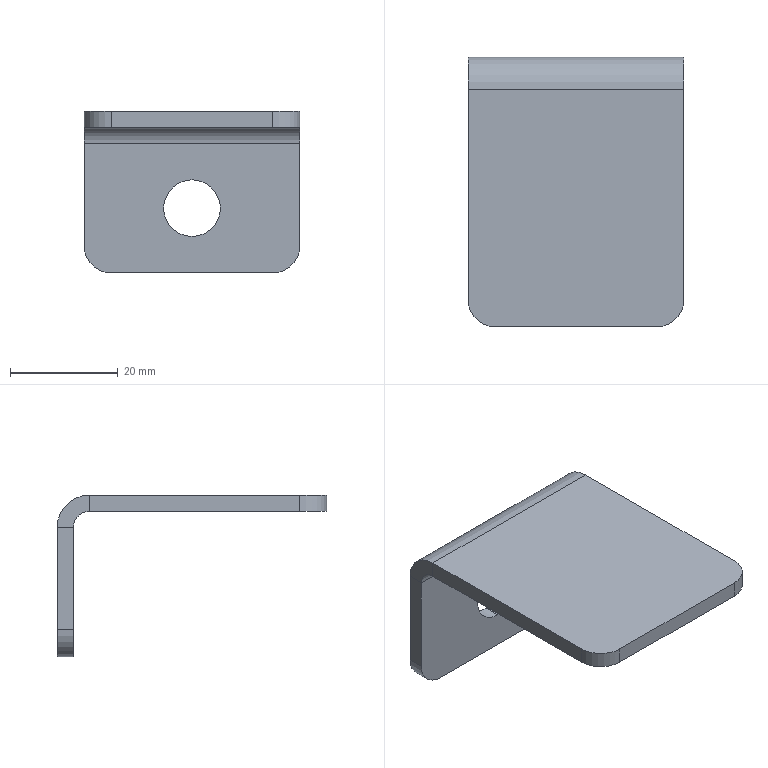Part | SolidWorks | features EdgeFlange 1, Fillet 1, FlatPattern 1, ICE 1, SMBaseFlange 1, SheetMetal 1 | 1 solid | 20 faces | box 40 x 50 x 30 mm | volume 8684 mm3 | plane 12 | cylinder 8 | commonest cylinder face diameters 10 x4 10.5 x2 6 x1 12 x1
STEP:
#1=CARTESIAN_POINT('',(0.,22.,-23.25));
#2=VERTEX_POINT('',#1);
#3=CARTESIAN_POINT('',(0.,22.,-12.75));
#4=VERTEX_POINT('',#3);
#5=CARTESIAN_POINT('',(0.,22.,-18.));
#6=DIRECTION('',(0.,1.,0.));
#7=DIRECTION('',(0.,0.,1.));
#8=AXIS2_PLACEMENT_3D('',#5,#6,#7);
#9=CIRCLE('',#8,5.25);
#10=EDGE_CURVE('',#2,#4,#9,.T.);
#11=ORIENTED_EDGE('',*,*,#10,.F.);
#12=CARTESIAN_POINT('',(0.,25.,-23.25));
#13=VERTEX_POINT('',#12);
#14=CARTESIAN_POINT('',(0.,15.,-23.25));
#15=DIRECTION('',(0.,1.,0.));
#16=VECTOR('',#15,1000.);
#17=LINE('',#14,#16);
#18=EDGE_CURVE('',#2,#13,#17,.T.);
#19=ORIENTED_EDGE('',*,*,#18,.T.);
#20=CARTESIAN_POINT('',(0.,25.,-12.75));
#21=VERTEX_POINT('',#20);
#22=CARTESIAN_POINT('',(0.,25.,-18.));
#23=DIRECTION('',(0.,1.,0.));
#24=DIRECTION('',(0.,0.,1.));
#25=AXIS2_PLACEMENT_3D('',#22,#23,#24);
#26=CIRCLE('',#25,5.25);
#27=EDGE_CURVE('',#13,#21,#26,.T.);
#28=ORIENTED_EDGE('',*,*,#27,.T.);
#29=CARTESIAN_POINT('',(0.,15.,-12.75));
#30=DIRECTION('',(0.,1.,0.));
#31=VECTOR('',#30,1000.);
#32=LINE('',#29,#31);
#33=EDGE_CURVE('',#4,#21,#32,.T.);
#34=ORIENTED_EDGE('',*,*,#33,.F.);
#35=EDGE_LOOP('',(#11,#19,#28,#34));
#36=FACE_OUTER_BOUND('',#35,.T.);
#37=CARTESIAN_POINT('',(0.,15.,-18.));
#38=DIRECTION('',(0.,1.,0.));
#39=DIRECTION('',(0.,0.,1.));
#40=AXIS2_PLACEMENT_3D('',#37,#38,#39);
#41=CYLINDRICAL_SURFACE('',#40,5.25);
#42=ADVANCED_FACE('',(#36),#41,.F.);
#43=CARTESIAN_POINT('',(20.,-20.,0.));
#44=VERTEX_POINT('',#43);
#45=CARTESIAN_POINT('',(20.,19.,0.));
#46=VERTEX_POINT('',#45);
#47=CARTESIAN_POINT('',(20.,25.,0.));
#48=DIRECTION('',(0.,1.,0.));
#49=VECTOR('',#48,1000.);
#50=LINE('',#47,#49);
#51=EDGE_CURVE('',#44,#46,#50,.T.);
#52=ORIENTED_EDGE('',*,*,#51,.F.);
#53=CARTESIAN_POINT('',(20.,-20.,-3.));
#54=VERTEX_POINT('',#53);
#55=CARTESIAN_POINT('',(20.,-20.,-3.));
#56=DIRECTION('',(0.,0.,-1.));
#57=VECTOR('',#56,1000.);
#58=LINE('',#55,#57);
#59=EDGE_CURVE('',#44,#54,#58,.T.);
#60=ORIENTED_EDGE('',*,*,#59,.T.);
#61=CARTESIAN_POINT('',(20.,19.,-3.));
#62=VERTEX_POINT('',#61);
#63=CARTESIAN_POINT('',(20.,25.,-3.));
#64=DIRECTION('',(0.,1.,0.));
#65=VECTOR('',#64,1000.);
#66=LINE('',#63,#65);
#67=EDGE_CURVE('',#54,#62,#66,.T.);
#68=ORIENTED_EDGE('',*,*,#67,.T.);
#69=CARTESIAN_POINT('',(20.,19.,-3.));
#70=DIRECTION('',(0.,0.,1.));
#71=VECTOR('',#70,1000.);
#72=LINE('',#69,#71);
#73=EDGE_CURVE('',#62,#46,#72,.T.);
#74=ORIENTED_EDGE('',*,*,#73,.T.);
#75=EDGE_LOOP('',(#52,#60,#68,#74));
#76=FACE_OUTER_BOUND('',#75,.T.);
#77=CARTESIAN_POINT('',(20.,25.,-3.));
#78=DIRECTION('',(1.,0.,0.));
#79=DIRECTION('',(0.,1.,0.));
#80=AXIS2_PLACEMENT_3D('',#77,#78,#79);
#81=PLANE('',#80);
#82=ADVANCED_FACE('',(#76),#81,.T.);
#83=CARTESIAN_POINT('',(-15.,-25.,-3.));
#84=VERTEX_POINT('',#83);
#85=CARTESIAN_POINT('',(15.,-25.,-3.));
#86=VERTEX_POINT('',#85);
#87=CARTESIAN_POINT('',(-20.,-25.,-3.));
#88=DIRECTION('',(1.,0.,0.));
#89=VECTOR('',#88,1000.);
#90=LINE('',#87,#89);
#91=EDGE_CURVE('',#84,#86,#90,.T.);
#92=ORIENTED_EDGE('',*,*,#91,.F.);
#93=CARTESIAN_POINT('',(-20.,-20.,-3.));
#94=VERTEX_POINT('',#93);
#95=CARTESIAN_POINT('',(-15.,-20.,-3.));
#96=DIRECTION('',(0.,0.,-1.));
#97=DIRECTION('',(1.,0.,0.));
#98=AXIS2_PLACEMENT_3D('',#95,#96,#97);
#99=CIRCLE('',#98,5.);
#100=EDGE_CURVE('',#84,#94,#99,.T.);
#101=ORIENTED_EDGE('',*,*,#100,.T.);
#102=CARTESIAN_POINT('',(-20.,19.,-3.));
#103=VERTEX_POINT('',#102);
#104=CARTESIAN_POINT('',(-20.,25.,-3.));
#105=DIRECTION('',(0.,-1.,0.));
#106=VECTOR('',#105,1000.);
#107=LINE('',#104,#106);
#108=EDGE_CURVE('',#103,#94,#107,.T.);
#109=ORIENTED_EDGE('',*,*,#108,.F.);
#110=CARTESIAN_POINT('',(20.,19.,-3.));
#111=DIRECTION('',(-1.,0.,0.));
#112=VECTOR('',#111,1000.);
#113=LINE('',#110,#112);
#114=EDGE_CURVE('',#62,#103,#113,.T.);
#115=ORIENTED_EDGE('',*,*,#114,.F.);
#116=ORIENTED_EDGE('',*,*,#67,.F.);
#117=CARTESIAN_POINT('',(15.,-20.,-3.));
#118=DIRECTION('',(0.,0.,-1.));
#119=DIRECTION('',(1.,0.,0.));
#120=AXIS2_PLACEMENT_3D('',#117,#118,#119);
#121=CIRCLE('',#120,5.);
#122=EDGE_CURVE('',#54,#86,#121,.T.);
#123=ORIENTED_EDGE('',*,*,#122,.T.);
#124=EDGE_LOOP('',(#92,#101,#109,#115,#116,#123));
#125=FACE_OUTER_BOUND('',#124,.T.);
#126=CARTESIAN_POINT('',(0.,0.,-3.));
#127=DIRECTION('',(0.,0.,1.));
#128=DIRECTION('',(1.,0.,0.));
#129=AXIS2_PLACEMENT_3D('',#126,#127,#128);
#130=PLANE('',#129);
#131=ADVANCED_FACE('',(#125),#130,.F.);
#132=CARTESIAN_POINT('',(-20.,19.,0.));
#133=VERTEX_POINT('',#132);
#134=CARTESIAN_POINT('',(-20.,-20.,0.));
#135=VERTEX_POINT('',#134);
#136=CARTESIAN_POINT('',(-20.,25.,0.));
#137=DIRECTION('',(0.,-1.,0.));
#138=VECTOR('',#137,1000.);
#139=LINE('',#136,#138);
#140=EDGE_CURVE('',#133,#135,#139,.T.);
#141=ORIENTED_EDGE('',*,*,#140,.T.);
#142=CARTESIAN_POINT('',(-15.,-25.,0.));
#143=VERTEX_POINT('',#142);
#144=CARTESIAN_POINT('',(-15.,-20.,0.));
#145=DIRECTION('',(0.,0.,1.));
#146=DIRECTION('',(1.,0.,0.));
#147=AXIS2_PLACEMENT_3D('',#144,#145,#146);
#148=CIRCLE('',#147,5.);
#149=EDGE_CURVE('',#135,#143,#148,.T.);
#150=ORIENTED_EDGE('',*,*,#149,.T.);
#151=CARTESIAN_POINT('',(15.,-25.,0.));
#152=VERTEX_POINT('',#151);
#153=CARTESIAN_POINT('',(-20.,-25.,0.));
#154=DIRECTION('',(1.,0.,0.));
#155=VECTOR('',#154,1000.);
#156=LINE('',#153,#155);
#157=EDGE_CURVE('',#143,#152,#156,.T.);
#158=ORIENTED_EDGE('',*,*,#157,.T.);
#159=CARTESIAN_POINT('',(15.,-20.,0.));
#160=DIRECTION('',(0.,0.,1.));
#161=DIRECTION('',(1.,0.,0.));
#162=AXIS2_PLACEMENT_3D('',#159,#160,#161);
#163=CIRCLE('',#162,5.);
#164=EDGE_CURVE('',#152,#44,#163,.T.);
#165=ORIENTED_EDGE('',*,*,#164,.T.);
#166=ORIENTED_EDGE('',*,*,#51,.T.);
#167=CARTESIAN_POINT('',(20.,19.,0.));
#168=DIRECTION('',(-1.,0.,0.));
#169=VECTOR('',#168,1000.);
#170=LINE('',#167,#169);
#171=EDGE_CURVE('',#46,#133,#170,.T.);
#172=ORIENTED_EDGE('',*,*,#171,.T.);
#173=EDGE_LOOP('',(#141,#150,#158,#165,#166,#172));
#174=FACE_OUTER_BOUND('',#173,.T.);
#175=CARTESIAN_POINT('',(0.,0.,0.));
#176=DIRECTION('',(0.,0.,1.));
#177=DIRECTION('',(1.,0.,0.));
#178=AXIS2_PLACEMENT_3D('',#175,#176,#177);
#179=PLANE('',#178);
#180=ADVANCED_FACE('',(#174),#179,.T.);
#181=ORIENTED_EDGE('',*,*,#157,.F.);
#182=CARTESIAN_POINT('',(-15.,-25.,-3.));
#183=DIRECTION('',(0.,0.,-1.));
#184=VECTOR('',#183,1000.);
#185=LINE('',#182,#184);
#186=EDGE_CURVE('',#143,#84,#185,.T.);
#187=ORIENTED_EDGE('',*,*,#186,.T.);
#188=ORIENTED_EDGE('',*,*,#91,.T.);
#189=CARTESIAN_POINT('',(15.,-25.,-3.));
#190=DIRECTION('',(0.,0.,1.));
#191=VECTOR('',#190,1000.);
#192=LINE('',#189,#191);
#193=EDGE_CURVE('',#86,#152,#192,.T.);
#194=ORIENTED_EDGE('',*,*,#193,.T.);
#195=EDGE_LOOP('',(#181,#187,#188,#194));
#196=FACE_OUTER_BOUND('',#195,.T.);
#197=CARTESIAN_POINT('',(-20.,-25.,-3.));
#198=DIRECTION('',(0.,-1.,0.));
#199=DIRECTION('',(0.,0.,-1.));
#200=AXIS2_PLACEMENT_3D('',#197,#198,#199);
#201=PLANE('',#200);
#202=ADVANCED_FACE('',(#196),#201,.T.);
#203=ORIENTED_EDGE('',*,*,#108,.T.);
#204=CARTESIAN_POINT('',(-20.,-20.,-3.));
#205=DIRECTION('',(0.,0.,1.));
#206=VECTOR('',#205,1000.);
#207=LINE('',#204,#206);
#208=EDGE_CURVE('',#94,#135,#207,.T.);
#209=ORIENTED_EDGE('',*,*,#208,.T.);
#210=ORIENTED_EDGE('',*,*,#140,.F.);
#211=CARTESIAN_POINT('',(-20.,19.,-3.));
#212=DIRECTION('',(0.,0.,1.));
#213=VECTOR('',#212,1000.);
#214=LINE('',#211,#213);
#215=EDGE_CURVE('',#103,#133,#214,.T.);
#216=ORIENTED_EDGE('',*,*,#215,.F.);
#217=EDGE_LOOP('',(#203,#209,#210,#216));
#218=FACE_OUTER_BOUND('',#217,.T.);
#219=CARTESIAN_POINT('',(-20.,25.,-3.));
#220=DIRECTION('',(-1.,0.,0.));
#221=DIRECTION('',(0.,-1.,0.));
#222=AXIS2_PLACEMENT_3D('',#219,#220,#221);
#223=PLANE('',#222);
#224=ADVANCED_FACE('',(#218),#223,.T.);
#225=CARTESIAN_POINT('',(-20.,22.,-6.));
#226=VERTEX_POINT('',#225);
#227=CARTESIAN_POINT('',(-20.,25.,-6.));
#228=VERTEX_POINT('',#227);
#229=CARTESIAN_POINT('',(-20.,25.,-6.));
#230=DIRECTION('',(0.,1.,0.));
#231=VECTOR('',#230,1000.);
#232=LINE('',#229,#231);
#233=EDGE_CURVE('',#226,#228,#232,.T.);
#234=ORIENTED_EDGE('',*,*,#233,.F.);
#235=CARTESIAN_POINT('',(-20.,19.,-6.));
#236=DIRECTION('',(-1.,0.,0.));
#237=DIRECTION('',(0.,0.,-1.));
#238=AXIS2_PLACEMENT_3D('',#235,#236,#237);
#239=CIRCLE('',#238,3.);
#240=EDGE_CURVE('',#103,#226,#239,.T.);
#241=ORIENTED_EDGE('',*,*,#240,.F.);
#242=ORIENTED_EDGE('',*,*,#215,.T.);
#243=CARTESIAN_POINT('',(-20.,19.,-6.));
#244=DIRECTION('',(-1.,0.,0.));
#245=DIRECTION('',(0.,0.,-1.));
#246=AXIS2_PLACEMENT_3D('',#243,#244,#245);
#247=CIRCLE('',#246,6.);
#248=EDGE_CURVE('',#133,#228,#247,.T.);
#249=ORIENTED_EDGE('',*,*,#248,.T.);
#250=EDGE_LOOP('',(#234,#241,#242,#249));
#251=FACE_OUTER_BOUND('',#250,.T.);
#252=CARTESIAN_POINT('',(-20.,19.,-6.));
#253=DIRECTION('',(-1.,0.,0.));
#254=DIRECTION('',(0.,0.,1.));
#255=AXIS2_PLACEMENT_3D('',#252,#253,#254);
#256=PLANE('',#255);
#257=ADVANCED_FACE('',(#251),#256,.T.);
#258=CARTESIAN_POINT('',(20.,22.,-6.));
#259=VERTEX_POINT('',#258);
#260=CARTESIAN_POINT('',(20.,19.,-6.));
#261=DIRECTION('',(1.,0.,0.));
#262=DIRECTION('',(0.,0.,-1.));
#263=AXIS2_PLACEMENT_3D('',#260,#261,#262);
#264=CIRCLE('',#263,3.);
#265=EDGE_CURVE('',#259,#62,#264,.T.);
#266=ORIENTED_EDGE('',*,*,#265,.F.);
#267=CARTESIAN_POINT('',(20.,25.,-6.));
#268=VERTEX_POINT('',#267);
#269=CARTESIAN_POINT('',(20.,22.,-6.));
#270=DIRECTION('',(0.,1.,0.));
#271=VECTOR('',#270,1000.);
#272=LINE('',#269,#271);
#273=EDGE_CURVE('',#259,#268,#272,.T.);
#274=ORIENTED_EDGE('',*,*,#273,.T.);
#275=CARTESIAN_POINT('',(20.,19.,-6.));
#276=DIRECTION('',(1.,0.,0.));
#277=DIRECTION('',(0.,0.,-1.));
#278=AXIS2_PLACEMENT_3D('',#275,#276,#277);
#279=CIRCLE('',#278,6.);
#280=EDGE_CURVE('',#268,#46,#279,.T.);
#281=ORIENTED_EDGE('',*,*,#280,.T.);
#282=ORIENTED_EDGE('',*,*,#73,.F.);
#283=EDGE_LOOP('',(#266,#274,#281,#282));
#284=FACE_OUTER_BOUND('',#283,.T.);
#285=CARTESIAN_POINT('',(20.,19.,-6.));
#286=DIRECTION('',(-1.,0.,0.));
#287=DIRECTION('',(0.,0.,1.));
#288=AXIS2_PLACEMENT_3D('',#285,#286,#287);
#289=PLANE('',#288);
#290=ADVANCED_FACE('',(#284),#289,.F.);
#291=ORIENTED_EDGE('',*,*,#171,.F.);
#292=ORIENTED_EDGE('',*,*,#280,.F.);
#293=CARTESIAN_POINT('',(0.,25.,-6.));
#294=DIRECTION('',(1.,0.,0.));
#295=VECTOR('',#294,1000.);
#296=LINE('',#293,#295);
#297=EDGE_CURVE('',#228,#268,#296,.T.);
#298=ORIENTED_EDGE('',*,*,#297,.F.);
#299=ORIENTED_EDGE('',*,*,#248,.F.);
#300=EDGE_LOOP('',(#291,#292,#298,#299));
#301=FACE_OUTER_BOUND('',#300,.T.);
#302=CARTESIAN_POINT('',(20.,19.,-6.));
#303=DIRECTION('',(1.,0.,0.));
#304=DIRECTION('',(0.,1.,0.));
#305=AXIS2_PLACEMENT_3D('',#302,#303,#304);
#306=CYLINDRICAL_SURFACE('',#305,6.);
#307=ADVANCED_FACE('',(#301),#306,.T.);
#308=ORIENTED_EDGE('',*,*,#114,.T.);
#309=ORIENTED_EDGE('',*,*,#240,.T.);
#310=CARTESIAN_POINT('',(-20.,22.,-6.));
#311=DIRECTION('',(1.,0.,0.));
#312=VECTOR('',#311,1000.);
#313=LINE('',#310,#312);
#314=EDGE_CURVE('',#226,#259,#313,.T.);
#315=ORIENTED_EDGE('',*,*,#314,.T.);
#316=ORIENTED_EDGE('',*,*,#265,.T.);
#317=EDGE_LOOP('',(#308,#309,#315,#316));
#318=FACE_OUTER_BOUND('',#317,.T.);
#319=CARTESIAN_POINT('',(20.,19.,-6.));
#320=DIRECTION('',(1.,0.,0.));
#321=DIRECTION('',(0.,1.,0.));
#322=AXIS2_PLACEMENT_3D('',#319,#320,#321);
#323=CYLINDRICAL_SURFACE('',#322,3.);
#324=ADVANCED_FACE('',(#318),#323,.F.);
#325=CARTESIAN_POINT('',(20.,22.,-25.));
#326=VERTEX_POINT('',#325);
#327=CARTESIAN_POINT('',(20.,22.,0.));
#328=DIRECTION('',(0.,0.,1.));
#329=VECTOR('',#328,1000.);
#330=LINE('',#327,#329);
#331=EDGE_CURVE('',#326,#259,#330,.T.);
#332=ORIENTED_EDGE('',*,*,#331,.F.);
#333=CARTESIAN_POINT('',(20.,25.,-25.));
#334=VERTEX_POINT('',#333);
#335=CARTESIAN_POINT('',(20.,25.,-25.));
#336=DIRECTION('',(0.,1.,0.));
#337=VECTOR('',#336,1000.);
#338=LINE('',#335,#337);
#339=EDGE_CURVE('',#326,#334,#338,.T.);
#340=ORIENTED_EDGE('',*,*,#339,.T.);
#341=CARTESIAN_POINT('',(20.,25.,-3.));
#342=DIRECTION('',(0.,0.,1.));
#343=VECTOR('',#342,1000.);
#344=LINE('',#341,#343);
#345=EDGE_CURVE('',#334,#268,#344,.T.);
#346=ORIENTED_EDGE('',*,*,#345,.T.);
#347=ORIENTED_EDGE('',*,*,#273,.F.);
#348=EDGE_LOOP('',(#332,#340,#346,#347));
#349=FACE_OUTER_BOUND('',#348,.T.);
#350=CARTESIAN_POINT('',(20.,25.,-3.));
#351=DIRECTION('',(1.,0.,0.));
#352=DIRECTION('',(0.,0.,-1.));
#353=AXIS2_PLACEMENT_3D('',#350,#351,#352);
#354=PLANE('',#353);
#355=ADVANCED_FACE('',(#349),#354,.T.);
#356=CARTESIAN_POINT('',(-20.,25.,-25.));
#357=VERTEX_POINT('',#356);
#358=CARTESIAN_POINT('',(-20.,25.,-30.));
#359=DIRECTION('',(0.,0.,-1.));
#360=VECTOR('',#359,1000.);
#361=LINE('',#358,#360);
#362=EDGE_CURVE('',#228,#357,#361,.T.);
#363=ORIENTED_EDGE('',*,*,#362,.T.);
#364=CARTESIAN_POINT('',(-20.,22.,-25.));
#365=VERTEX_POINT('',#364);
#366=CARTESIAN_POINT('',(-20.,25.,-25.));
#367=DIRECTION('',(0.,-1.,0.));
#368=VECTOR('',#367,1000.);
#369=LINE('',#366,#368);
#370=EDGE_CURVE('',#357,#365,#369,.T.);
#371=ORIENTED_EDGE('',*,*,#370,.T.);
#372=CARTESIAN_POINT('',(-20.,22.,0.));
#373=DIRECTION('',(0.,0.,-1.));
#374=VECTOR('',#373,1000.);
#375=LINE('',#372,#374);
#376=EDGE_CURVE('',#226,#365,#375,.T.);
#377=ORIENTED_EDGE('',*,*,#376,.F.);
#378=ORIENTED_EDGE('',*,*,#233,.T.);
#379=EDGE_LOOP('',(#363,#371,#377,#378));
#380=FACE_OUTER_BOUND('',#379,.T.);
#381=CARTESIAN_POINT('',(-20.,25.,-30.));
#382=DIRECTION('',(-1.,0.,0.));
#383=DIRECTION('',(0.,0.,1.));
#384=AXIS2_PLACEMENT_3D('',#381,#382,#383);
#385=PLANE('',#384);
#386=ADVANCED_FACE('',(#380),#385,.T.);
#387=CARTESIAN_POINT('',(0.,25.,-18.));
#388=DIRECTION('',(0.,1.,0.));
#389=DIRECTION('',(0.,0.,1.));
#390=AXIS2_PLACEMENT_3D('',#387,#388,#389);
#391=CIRCLE('',#390,5.25);
#392=EDGE_CURVE('',#21,#13,#391,.T.);
#393=ORIENTED_EDGE('',*,*,#392,.F.);
#394=ORIENTED_EDGE('',*,*,#27,.F.);
#395=EDGE_LOOP('',(#393,#394));
#396=FACE_BOUND('',#395,.T.);
#397=ORIENTED_EDGE('',*,*,#345,.F.);
#398=CARTESIAN_POINT('',(15.,25.,-30.));
#399=VERTEX_POINT('',#398);
#400=CARTESIAN_POINT('',(15.,25.,-25.));
#401=DIRECTION('',(0.,1.,0.));
#402=DIRECTION('',(0.,0.,1.));
#403=AXIS2_PLACEMENT_3D('',#400,#401,#402);
#404=CIRCLE('',#403,5.);
#405=EDGE_CURVE('',#334,#399,#404,.T.);
#406=ORIENTED_EDGE('',*,*,#405,.T.);
#407=CARTESIAN_POINT('',(-15.,25.,-30.));
#408=VERTEX_POINT('',#407);
#409=CARTESIAN_POINT('',(20.,25.,-30.));
#410=DIRECTION('',(1.,0.,0.));
#411=VECTOR('',#410,1000.);
#412=LINE('',#409,#411);
#413=EDGE_CURVE('',#408,#399,#412,.T.);
#414=ORIENTED_EDGE('',*,*,#413,.F.);
#415=CARTESIAN_POINT('',(-15.,25.,-25.));
#416=DIRECTION('',(0.,1.,0.));
#417=DIRECTION('',(0.,0.,1.));
#418=AXIS2_PLACEMENT_3D('',#415,#416,#417);
#419=CIRCLE('',#418,5.);
#420=EDGE_CURVE('',#408,#357,#419,.T.);
#421=ORIENTED_EDGE('',*,*,#420,.T.);
#422=ORIENTED_EDGE('',*,*,#362,.F.);
#423=ORIENTED_EDGE('',*,*,#297,.T.);
#424=EDGE_LOOP('',(#397,#406,#414,#421,#422,#423));
#425=FACE_OUTER_BOUND('',#424,.T.);
#426=CARTESIAN_POINT('',(0.,25.,0.));
#427=DIRECTION('',(0.,1.,0.));
#428=DIRECTION('',(0.,0.,1.));
#429=AXIS2_PLACEMENT_3D('',#426,#427,#428);
#430=PLANE('',#429);
#431=ADVANCED_FACE('',(#396,#425),#430,.T.);
#432=CARTESIAN_POINT('',(0.,22.,-18.));
#433=DIRECTION('',(0.,1.,0.));
#434=DIRECTION('',(0.,0.,1.));
#435=AXIS2_PLACEMENT_3D('',#432,#433,#434);
#436=CIRCLE('',#435,5.25);
#437=EDGE_CURVE('',#4,#2,#436,.T.);
#438=ORIENTED_EDGE('',*,*,#437,.T.);
#439=ORIENTED_EDGE('',*,*,#10,.T.);
#440=EDGE_LOOP('',(#438,#439));
#441=FACE_BOUND('',#440,.T.);
#442=CARTESIAN_POINT('',(-15.,22.,-30.));
#443=VERTEX_POINT('',#442);
#444=CARTESIAN_POINT('',(15.,22.,-30.));
#445=VERTEX_POINT('',#444);
#446=CARTESIAN_POINT('',(0.,22.,-30.));
#447=DIRECTION('',(1.,0.,0.));
#448=VECTOR('',#447,1000.);
#449=LINE('',#446,#448);
#450=EDGE_CURVE('',#443,#445,#449,.T.);
#451=ORIENTED_EDGE('',*,*,#450,.T.);
#452=CARTESIAN_POINT('',(15.,22.,-25.));
#453=DIRECTION('',(0.,-1.,0.));
#454=DIRECTION('',(0.,0.,1.));
#455=AXIS2_PLACEMENT_3D('',#452,#453,#454);
#456=CIRCLE('',#455,5.);
#457=EDGE_CURVE('',#445,#326,#456,.T.);
#458=ORIENTED_EDGE('',*,*,#457,.T.);
#459=ORIENTED_EDGE('',*,*,#331,.T.);
#460=ORIENTED_EDGE('',*,*,#314,.F.);
#461=ORIENTED_EDGE('',*,*,#376,.T.);
#462=CARTESIAN_POINT('',(-15.,22.,-25.));
#463=DIRECTION('',(0.,-1.,0.));
#464=DIRECTION('',(0.,0.,1.));
#465=AXIS2_PLACEMENT_3D('',#462,#463,#464);
#466=CIRCLE('',#465,5.);
#467=EDGE_CURVE('',#365,#443,#466,.T.);
#468=ORIENTED_EDGE('',*,*,#467,.T.);
#469=EDGE_LOOP('',(#451,#458,#459,#460,#461,#468));
#470=FACE_OUTER_BOUND('',#469,.T.);
#471=CARTESIAN_POINT('',(0.,22.,0.));
#472=DIRECTION('',(0.,1.,0.));
#473=DIRECTION('',(0.,0.,1.));
#474=AXIS2_PLACEMENT_3D('',#471,#472,#473);
#475=PLANE('',#474);
#476=ADVANCED_FACE('',(#441,#470),#475,.F.);
#477=ORIENTED_EDGE('',*,*,#413,.T.);
#478=CARTESIAN_POINT('',(15.,25.,-30.));
#479=DIRECTION('',(0.,-1.,0.));
#480=VECTOR('',#479,1000.);
#481=LINE('',#478,#480);
#482=EDGE_CURVE('',#399,#445,#481,.T.);
#483=ORIENTED_EDGE('',*,*,#482,.T.);
#484=ORIENTED_EDGE('',*,*,#450,.F.);
#485=CARTESIAN_POINT('',(-15.,25.,-30.));
#486=DIRECTION('',(0.,1.,0.));
#487=VECTOR('',#486,1000.);
#488=LINE('',#485,#487);
#489=EDGE_CURVE('',#443,#408,#488,.T.);
#490=ORIENTED_EDGE('',*,*,#489,.T.);
#491=EDGE_LOOP('',(#477,#483,#484,#490));
#492=FACE_OUTER_BOUND('',#491,.T.);
#493=CARTESIAN_POINT('',(20.,25.,-30.));
#494=DIRECTION('',(0.,0.,-1.));
#495=DIRECTION('',(0.,1.,0.));
#496=AXIS2_PLACEMENT_3D('',#493,#494,#495);
#497=PLANE('',#496);
#498=ADVANCED_FACE('',(#492),#497,.T.);
#499=ORIENTED_EDGE('',*,*,#405,.F.);
#500=ORIENTED_EDGE('',*,*,#339,.F.);
#501=ORIENTED_EDGE('',*,*,#457,.F.);
#502=ORIENTED_EDGE('',*,*,#482,.F.);
#503=EDGE_LOOP('',(#499,#500,#501,#502));
#504=FACE_OUTER_BOUND('',#503,.T.);
#505=CARTESIAN_POINT('',(15.,25.,-25.));
#506=DIRECTION('',(0.,-1.,0.));
#507=DIRECTION('',(0.,0.,-1.));
#508=AXIS2_PLACEMENT_3D('',#505,#506,#507);
#509=CYLINDRICAL_SURFACE('',#508,5.);
#510=ADVANCED_FACE('',(#504),#509,.T.);
#511=ORIENTED_EDGE('',*,*,#420,.F.);
#512=ORIENTED_EDGE('',*,*,#489,.F.);
#513=ORIENTED_EDGE('',*,*,#467,.F.);
#514=ORIENTED_EDGE('',*,*,#370,.F.);
#515=EDGE_LOOP('',(#511,#512,#513,#514));
#516=FACE_OUTER_BOUND('',#515,.T.);
#517=CARTESIAN_POINT('',(-15.,25.,-25.));
#518=DIRECTION('',(0.,-1.,0.));
#519=DIRECTION('',(0.,0.,-1.));
#520=AXIS2_PLACEMENT_3D('',#517,#518,#519);
#521=CYLINDRICAL_SURFACE('',#520,5.);
#522=ADVANCED_FACE('',(#516),#521,.T.);
#523=ORIENTED_EDGE('',*,*,#100,.F.);
#524=ORIENTED_EDGE('',*,*,#186,.F.);
#525=ORIENTED_EDGE('',*,*,#149,.F.);
#526=ORIENTED_EDGE('',*,*,#208,.F.);
#527=EDGE_LOOP('',(#523,#524,#525,#526));
#528=FACE_OUTER_BOUND('',#527,.T.);
#529=CARTESIAN_POINT('',(-15.,-20.,-3.));
#530=DIRECTION('',(0.,0.,1.));
#531=DIRECTION('',(1.,0.,0.));
#532=AXIS2_PLACEMENT_3D('',#529,#530,#531);
#533=CYLINDRICAL_SURFACE('',#532,5.);
#534=ADVANCED_FACE('',(#528),#533,.T.);
#535=ORIENTED_EDGE('',*,*,#122,.F.);
#536=ORIENTED_EDGE('',*,*,#59,.F.);
#537=ORIENTED_EDGE('',*,*,#164,.F.);
#538=ORIENTED_EDGE('',*,*,#193,.F.);
#539=EDGE_LOOP('',(#535,#536,#537,#538));
#540=FACE_OUTER_BOUND('',#539,.T.);
#541=CARTESIAN_POINT('',(15.,-20.,-3.));
#542=DIRECTION('',(0.,0.,1.));
#543=DIRECTION('',(1.,0.,0.));
#544=AXIS2_PLACEMENT_3D('',#541,#542,#543);
#545=CYLINDRICAL_SURFACE('',#544,5.);
#546=ADVANCED_FACE('',(#540),#545,.T.);
#547=ORIENTED_EDGE('',*,*,#18,.F.);
#548=ORIENTED_EDGE('',*,*,#437,.F.);
#549=ORIENTED_EDGE('',*,*,#33,.T.);
#550=ORIENTED_EDGE('',*,*,#392,.T.);
#551=EDGE_LOOP('',(#547,#548,#549,#550));
#552=FACE_OUTER_BOUND('',#551,.T.);
#553=CARTESIAN_POINT('',(0.,15.,-18.));
#554=DIRECTION('',(0.,1.,0.));
#555=DIRECTION('',(0.,0.,1.));
#556=AXIS2_PLACEMENT_3D('',#553,#554,#555);
#557=CYLINDRICAL_SURFACE('',#556,5.25);
#558=ADVANCED_FACE('',(#552),#557,.F.);
#559=CLOSED_SHELL('',(#42,#82,#131,#180,#202,#224,#257,#290,#307,#324,#355,#386,#431,#476,#498,#510,#522,#534,#546,#558));
#560=MANIFOLD_SOLID_BREP('',#559);
#561=CARTESIAN_POINT('',(0.,0.,0.));
#562=DIRECTION('',(0.,0.,1.));
#563=DIRECTION('',(1.,0.,0.));
#564=AXIS2_PLACEMENT_3D('',#561,#562,#563);
#565=(LENGTH_UNIT()NAMED_UNIT(*)SI_UNIT(.MILLI.,.METRE.));
#566=UNCERTAINTY_MEASURE_WITH_UNIT(LENGTH_MEASURE(0.00001),#565,'','');
#567=(NAMED_UNIT(*)PLANE_ANGLE_UNIT()SI_UNIT($,.RADIAN.));
#568=(NAMED_UNIT(*)SI_UNIT($,.STERADIAN.)SOLID_ANGLE_UNIT());
#569=(GEOMETRIC_REPRESENTATION_CONTEXT(3)GLOBAL_UNCERTAINTY_ASSIGNED_CONTEXT((#566))GLOBAL_UNIT_ASSIGNED_CONTEXT((#565,#567,#568))REPRESENTATION_CONTEXT('',''));
#570=ADVANCED_BREP_SHAPE_REPRESENTATION('',(#560,#564),#569);